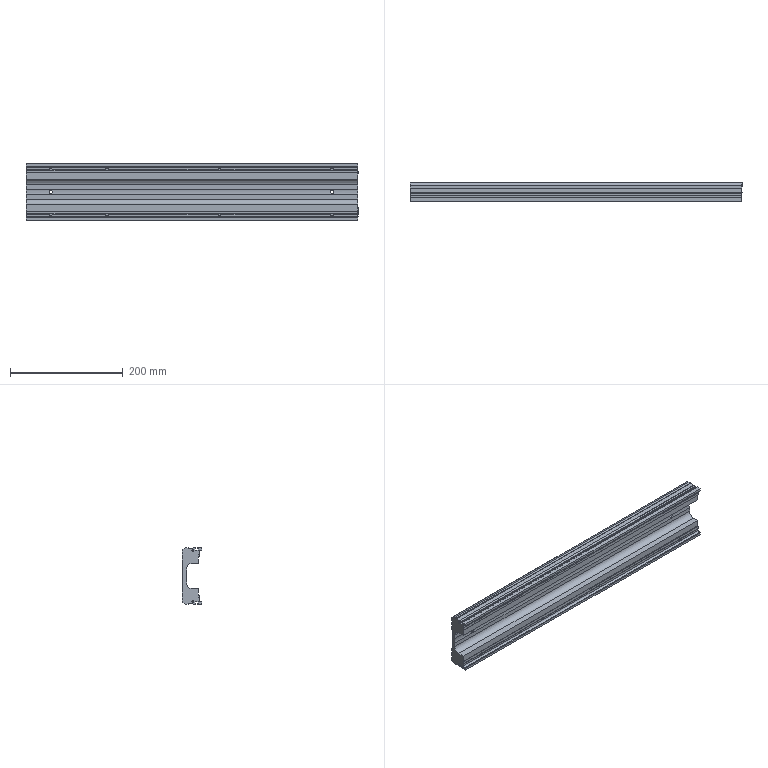Part | SolidWorks | features BaseBody 1 | 1 solid | 191 faces | box 590 x 35 x 100 mm | volume 1144362 mm3 | plane 121 | cylinder 70 | commonest cylinder face diameters 4.917 x32 8 x10 0.4 x8 0.6 x8 6 x6 3.2 x3